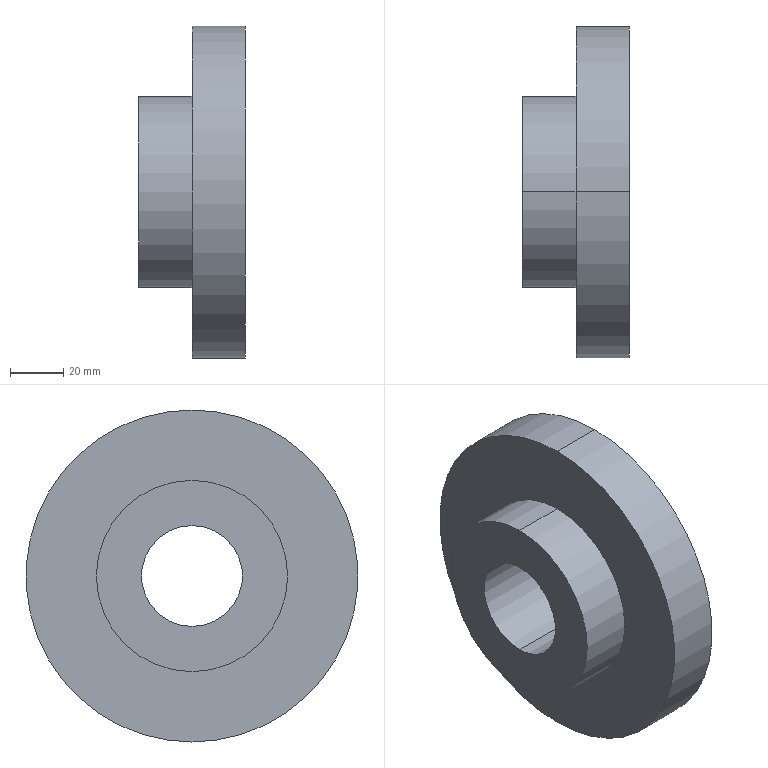Part | SolidWorks | features Revolution 1 | 1 solid | 9 faces | box 40 x 125 x 125 mm | volume 281502 mm3 | cylinder 6 | plane 3 | commonest cylinder face diameters 38 x2 72 x2 125 x2
STEP:
#1=CARTESIAN_POINT('',(40.,0.,62.5));
#2=VERTEX_POINT('',#1);
#3=CARTESIAN_POINT('',(40.,0.,-62.5));
#4=VERTEX_POINT('',#3);
#5=CARTESIAN_POINT('',(40.,0.,0.));
#6=DIRECTION('',(-1.,0.,0.));
#7=DIRECTION('',(0.,0.,1.));
#8=AXIS2_PLACEMENT_3D('',#5,#6,#7);
#9=CIRCLE('',#8,62.5);
#10=EDGE_CURVE('',#2,#4,#9,.T.);
#11=ORIENTED_EDGE('',*,*,#10,.T.);
#12=CARTESIAN_POINT('',(20.,0.,-62.5));
#13=VERTEX_POINT('',#12);
#14=CARTESIAN_POINT('',(0.,0.,-62.5));
#15=DIRECTION('',(-1.,0.,0.));
#16=VECTOR('',#15,1000.);
#17=LINE('',#14,#16);
#18=EDGE_CURVE('',#4,#13,#17,.T.);
#19=ORIENTED_EDGE('',*,*,#18,.T.);
#20=CARTESIAN_POINT('',(20.,0.,62.5));
#21=VERTEX_POINT('',#20);
#22=CARTESIAN_POINT('',(20.,0.,0.));
#23=DIRECTION('',(-1.,0.,0.));
#24=DIRECTION('',(0.,0.,1.));
#25=AXIS2_PLACEMENT_3D('',#22,#23,#24);
#26=CIRCLE('',#25,62.5);
#27=EDGE_CURVE('',#21,#13,#26,.T.);
#28=ORIENTED_EDGE('',*,*,#27,.F.);
#29=CARTESIAN_POINT('',(0.,0.,62.5));
#30=DIRECTION('',(-1.,0.,0.));
#31=VECTOR('',#30,1000.);
#32=LINE('',#29,#31);
#33=EDGE_CURVE('',#2,#21,#32,.T.);
#34=ORIENTED_EDGE('',*,*,#33,.F.);
#35=EDGE_LOOP('',(#11,#19,#28,#34));
#36=FACE_OUTER_BOUND('',#35,.T.);
#37=CARTESIAN_POINT('',(0.,0.,0.));
#38=DIRECTION('',(-1.,0.,0.));
#39=DIRECTION('',(0.,0.,1.));
#40=AXIS2_PLACEMENT_3D('',#37,#38,#39);
#41=CYLINDRICAL_SURFACE('',#40,62.5);
#42=ADVANCED_FACE('',(#36),#41,.T.);
#43=CARTESIAN_POINT('',(20.,0.,36.));
#44=VERTEX_POINT('',#43);
#45=CARTESIAN_POINT('',(20.,0.,-36.));
#46=VERTEX_POINT('',#45);
#47=CARTESIAN_POINT('',(20.,0.,0.));
#48=DIRECTION('',(-1.,0.,0.));
#49=DIRECTION('',(0.,0.,1.));
#50=AXIS2_PLACEMENT_3D('',#47,#48,#49);
#51=CIRCLE('',#50,36.);
#52=EDGE_CURVE('',#44,#46,#51,.T.);
#53=ORIENTED_EDGE('',*,*,#52,.T.);
#54=CARTESIAN_POINT('',(0.,0.,-36.));
#55=VERTEX_POINT('',#54);
#56=CARTESIAN_POINT('',(0.,0.,-36.));
#57=DIRECTION('',(-1.,0.,0.));
#58=VECTOR('',#57,1000.);
#59=LINE('',#56,#58);
#60=EDGE_CURVE('',#46,#55,#59,.T.);
#61=ORIENTED_EDGE('',*,*,#60,.T.);
#62=CARTESIAN_POINT('',(0.,0.,36.));
#63=VERTEX_POINT('',#62);
#64=CARTESIAN_POINT('',(0.,0.,0.));
#65=DIRECTION('',(-1.,0.,0.));
#66=DIRECTION('',(0.,0.,1.));
#67=AXIS2_PLACEMENT_3D('',#64,#65,#66);
#68=CIRCLE('',#67,36.);
#69=EDGE_CURVE('',#63,#55,#68,.T.);
#70=ORIENTED_EDGE('',*,*,#69,.F.);
#71=CARTESIAN_POINT('',(0.,0.,36.));
#72=DIRECTION('',(-1.,0.,0.));
#73=VECTOR('',#72,1000.);
#74=LINE('',#71,#73);
#75=EDGE_CURVE('',#44,#63,#74,.T.);
#76=ORIENTED_EDGE('',*,*,#75,.F.);
#77=EDGE_LOOP('',(#53,#61,#70,#76));
#78=FACE_OUTER_BOUND('',#77,.T.);
#79=CARTESIAN_POINT('',(0.,0.,0.));
#80=DIRECTION('',(-1.,0.,0.));
#81=DIRECTION('',(0.,0.,1.));
#82=AXIS2_PLACEMENT_3D('',#79,#80,#81);
#83=CYLINDRICAL_SURFACE('',#82,36.);
#84=ADVANCED_FACE('',(#78),#83,.T.);
#85=CARTESIAN_POINT('',(40.,0.,-19.));
#86=VERTEX_POINT('',#85);
#87=CARTESIAN_POINT('',(40.,0.,19.));
#88=VERTEX_POINT('',#87);
#89=CARTESIAN_POINT('',(40.,0.,0.));
#90=DIRECTION('',(-1.,0.,0.));
#91=DIRECTION('',(0.,0.,1.));
#92=AXIS2_PLACEMENT_3D('',#89,#90,#91);
#93=CIRCLE('',#92,19.);
#94=EDGE_CURVE('',#86,#88,#93,.T.);
#95=ORIENTED_EDGE('',*,*,#94,.F.);
#96=CARTESIAN_POINT('',(0.,0.,-19.));
#97=VERTEX_POINT('',#96);
#98=CARTESIAN_POINT('',(0.,0.,-19.));
#99=DIRECTION('',(-1.,0.,0.));
#100=VECTOR('',#99,1000.);
#101=LINE('',#98,#100);
#102=EDGE_CURVE('',#86,#97,#101,.T.);
#103=ORIENTED_EDGE('',*,*,#102,.T.);
#104=CARTESIAN_POINT('',(0.,0.,19.));
#105=VERTEX_POINT('',#104);
#106=CARTESIAN_POINT('',(0.,0.,0.));
#107=DIRECTION('',(-1.,0.,0.));
#108=DIRECTION('',(0.,0.,1.));
#109=AXIS2_PLACEMENT_3D('',#106,#107,#108);
#110=CIRCLE('',#109,19.);
#111=EDGE_CURVE('',#97,#105,#110,.T.);
#112=ORIENTED_EDGE('',*,*,#111,.T.);
#113=CARTESIAN_POINT('',(0.,0.,19.));
#114=DIRECTION('',(-1.,0.,0.));
#115=VECTOR('',#114,1000.);
#116=LINE('',#113,#115);
#117=EDGE_CURVE('',#88,#105,#116,.T.);
#118=ORIENTED_EDGE('',*,*,#117,.F.);
#119=EDGE_LOOP('',(#95,#103,#112,#118));
#120=FACE_OUTER_BOUND('',#119,.T.);
#121=CARTESIAN_POINT('',(0.,0.,0.));
#122=DIRECTION('',(-1.,0.,0.));
#123=DIRECTION('',(0.,0.,1.));
#124=AXIS2_PLACEMENT_3D('',#121,#122,#123);
#125=CYLINDRICAL_SURFACE('',#124,19.);
#126=ADVANCED_FACE('',(#120),#125,.F.);
#127=ORIENTED_EDGE('',*,*,#102,.F.);
#128=CARTESIAN_POINT('',(40.,0.,0.));
#129=DIRECTION('',(-1.,0.,0.));
#130=DIRECTION('',(0.,0.,1.));
#131=AXIS2_PLACEMENT_3D('',#128,#129,#130);
#132=CIRCLE('',#131,19.);
#133=EDGE_CURVE('',#88,#86,#132,.T.);
#134=ORIENTED_EDGE('',*,*,#133,.F.);
#135=ORIENTED_EDGE('',*,*,#117,.T.);
#136=CARTESIAN_POINT('',(0.,0.,0.));
#137=DIRECTION('',(-1.,0.,0.));
#138=DIRECTION('',(0.,0.,1.));
#139=AXIS2_PLACEMENT_3D('',#136,#137,#138);
#140=CIRCLE('',#139,19.);
#141=EDGE_CURVE('',#105,#97,#140,.T.);
#142=ORIENTED_EDGE('',*,*,#141,.T.);
#143=EDGE_LOOP('',(#127,#134,#135,#142));
#144=FACE_OUTER_BOUND('',#143,.T.);
#145=CARTESIAN_POINT('',(0.,0.,0.));
#146=DIRECTION('',(-1.,0.,0.));
#147=DIRECTION('',(0.,0.,1.));
#148=AXIS2_PLACEMENT_3D('',#145,#146,#147);
#149=CYLINDRICAL_SURFACE('',#148,19.);
#150=ADVANCED_FACE('',(#144),#149,.F.);
#151=ORIENTED_EDGE('',*,*,#69,.T.);
#152=CARTESIAN_POINT('',(0.,0.,0.));
#153=DIRECTION('',(-1.,0.,0.));
#154=DIRECTION('',(0.,0.,1.));
#155=AXIS2_PLACEMENT_3D('',#152,#153,#154);
#156=CIRCLE('',#155,36.);
#157=EDGE_CURVE('',#55,#63,#156,.T.);
#158=ORIENTED_EDGE('',*,*,#157,.T.);
#159=EDGE_LOOP('',(#151,#158));
#160=FACE_OUTER_BOUND('',#159,.T.);
#161=ORIENTED_EDGE('',*,*,#141,.F.);
#162=ORIENTED_EDGE('',*,*,#111,.F.);
#163=EDGE_LOOP('',(#161,#162));
#164=FACE_BOUND('',#163,.T.);
#165=CARTESIAN_POINT('',(0.,-19.,0.));
#166=DIRECTION('',(-1.,0.,0.));
#167=DIRECTION('',(0.,0.,1.));
#168=AXIS2_PLACEMENT_3D('',#165,#166,#167);
#169=PLANE('',#168);
#170=ADVANCED_FACE('',(#160,#164),#169,.T.);
#171=ORIENTED_EDGE('',*,*,#60,.F.);
#172=CARTESIAN_POINT('',(20.,0.,0.));
#173=DIRECTION('',(-1.,0.,0.));
#174=DIRECTION('',(0.,0.,1.));
#175=AXIS2_PLACEMENT_3D('',#172,#173,#174);
#176=CIRCLE('',#175,36.);
#177=EDGE_CURVE('',#46,#44,#176,.T.);
#178=ORIENTED_EDGE('',*,*,#177,.T.);
#179=ORIENTED_EDGE('',*,*,#75,.T.);
#180=ORIENTED_EDGE('',*,*,#157,.F.);
#181=EDGE_LOOP('',(#171,#178,#179,#180));
#182=FACE_OUTER_BOUND('',#181,.T.);
#183=CARTESIAN_POINT('',(0.,0.,0.));
#184=DIRECTION('',(-1.,0.,0.));
#185=DIRECTION('',(0.,0.,1.));
#186=AXIS2_PLACEMENT_3D('',#183,#184,#185);
#187=CYLINDRICAL_SURFACE('',#186,36.);
#188=ADVANCED_FACE('',(#182),#187,.T.);
#189=ORIENTED_EDGE('',*,*,#27,.T.);
#190=CARTESIAN_POINT('',(20.,0.,0.));
#191=DIRECTION('',(-1.,0.,0.));
#192=DIRECTION('',(0.,0.,1.));
#193=AXIS2_PLACEMENT_3D('',#190,#191,#192);
#194=CIRCLE('',#193,62.5);
#195=EDGE_CURVE('',#13,#21,#194,.T.);
#196=ORIENTED_EDGE('',*,*,#195,.T.);
#197=EDGE_LOOP('',(#189,#196));
#198=FACE_OUTER_BOUND('',#197,.T.);
#199=ORIENTED_EDGE('',*,*,#52,.F.);
#200=ORIENTED_EDGE('',*,*,#177,.F.);
#201=EDGE_LOOP('',(#199,#200));
#202=FACE_BOUND('',#201,.T.);
#203=CARTESIAN_POINT('',(20.,-36.,0.));
#204=DIRECTION('',(-1.,0.,0.));
#205=DIRECTION('',(0.,0.,1.));
#206=AXIS2_PLACEMENT_3D('',#203,#204,#205);
#207=PLANE('',#206);
#208=ADVANCED_FACE('',(#198,#202),#207,.T.);
#209=ORIENTED_EDGE('',*,*,#18,.F.);
#210=CARTESIAN_POINT('',(40.,0.,0.));
#211=DIRECTION('',(-1.,0.,0.));
#212=DIRECTION('',(0.,0.,1.));
#213=AXIS2_PLACEMENT_3D('',#210,#211,#212);
#214=CIRCLE('',#213,62.5);
#215=EDGE_CURVE('',#4,#2,#214,.T.);
#216=ORIENTED_EDGE('',*,*,#215,.T.);
#217=ORIENTED_EDGE('',*,*,#33,.T.);
#218=ORIENTED_EDGE('',*,*,#195,.F.);
#219=EDGE_LOOP('',(#209,#216,#217,#218));
#220=FACE_OUTER_BOUND('',#219,.T.);
#221=CARTESIAN_POINT('',(0.,0.,0.));
#222=DIRECTION('',(-1.,0.,0.));
#223=DIRECTION('',(0.,0.,1.));
#224=AXIS2_PLACEMENT_3D('',#221,#222,#223);
#225=CYLINDRICAL_SURFACE('',#224,62.5);
#226=ADVANCED_FACE('',(#220),#225,.T.);
#227=ORIENTED_EDGE('',*,*,#133,.T.);
#228=ORIENTED_EDGE('',*,*,#94,.T.);
#229=EDGE_LOOP('',(#227,#228));
#230=FACE_BOUND('',#229,.T.);
#231=ORIENTED_EDGE('',*,*,#10,.F.);
#232=ORIENTED_EDGE('',*,*,#215,.F.);
#233=EDGE_LOOP('',(#231,#232));
#234=FACE_OUTER_BOUND('',#233,.T.);
#235=CARTESIAN_POINT('',(40.,-62.5,0.));
#236=DIRECTION('',(1.,0.,0.));
#237=DIRECTION('',(0.,0.,-1.));
#238=AXIS2_PLACEMENT_3D('',#235,#236,#237);
#239=PLANE('',#238);
#240=ADVANCED_FACE('',(#230,#234),#239,.T.);
#241=CLOSED_SHELL('',(#42,#84,#126,#150,#170,#188,#208,#226,#240));
#242=MANIFOLD_SOLID_BREP('',#241);
#243=CARTESIAN_POINT('',(0.,0.,0.));
#244=DIRECTION('',(0.,0.,1.));
#245=DIRECTION('',(1.,0.,0.));
#246=AXIS2_PLACEMENT_3D('',#243,#244,#245);
#247=(LENGTH_UNIT()NAMED_UNIT(*)SI_UNIT(.MILLI.,.METRE.));
#248=UNCERTAINTY_MEASURE_WITH_UNIT(LENGTH_MEASURE(0.00001),#247,'','');
#249=(NAMED_UNIT(*)PLANE_ANGLE_UNIT()SI_UNIT($,.RADIAN.));
#250=(NAMED_UNIT(*)SI_UNIT($,.STERADIAN.)SOLID_ANGLE_UNIT());
#251=(GEOMETRIC_REPRESENTATION_CONTEXT(3)GLOBAL_UNCERTAINTY_ASSIGNED_CONTEXT((#248))GLOBAL_UNIT_ASSIGNED_CONTEXT((#247,#249,#250))REPRESENTATION_CONTEXT('',''));
#252=ADVANCED_BREP_SHAPE_REPRESENTATION('',(#242,#246),#251);